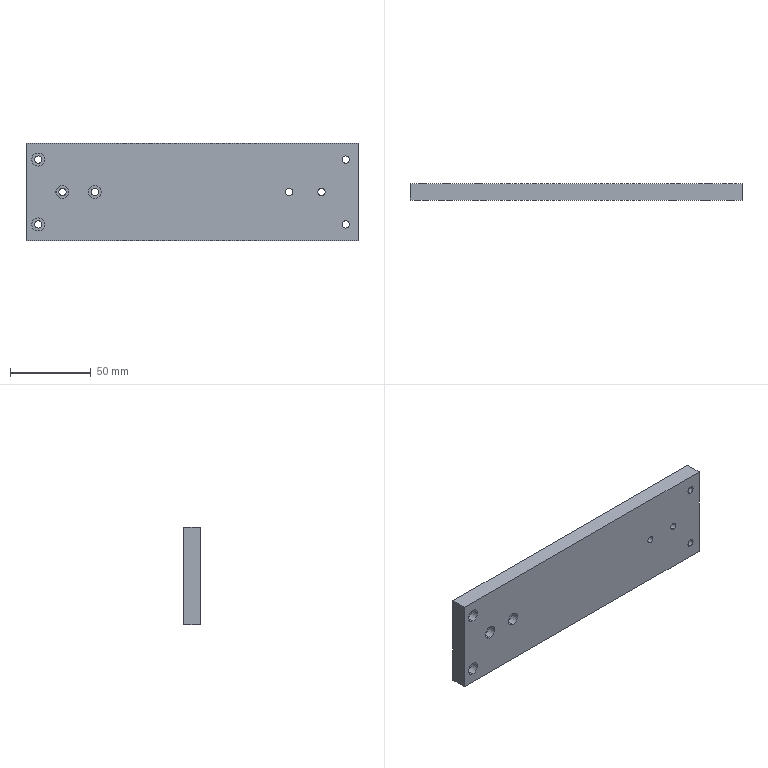Part | STEP file | Camera bracket top plate | 1 solid | 54 faces | box 205 x 10 x 60 mm | volume 120463 mm3 | cylinder 32 | plane 14 | cone 8 | commonest cylinder face diameters 4.5 x16 8 x16